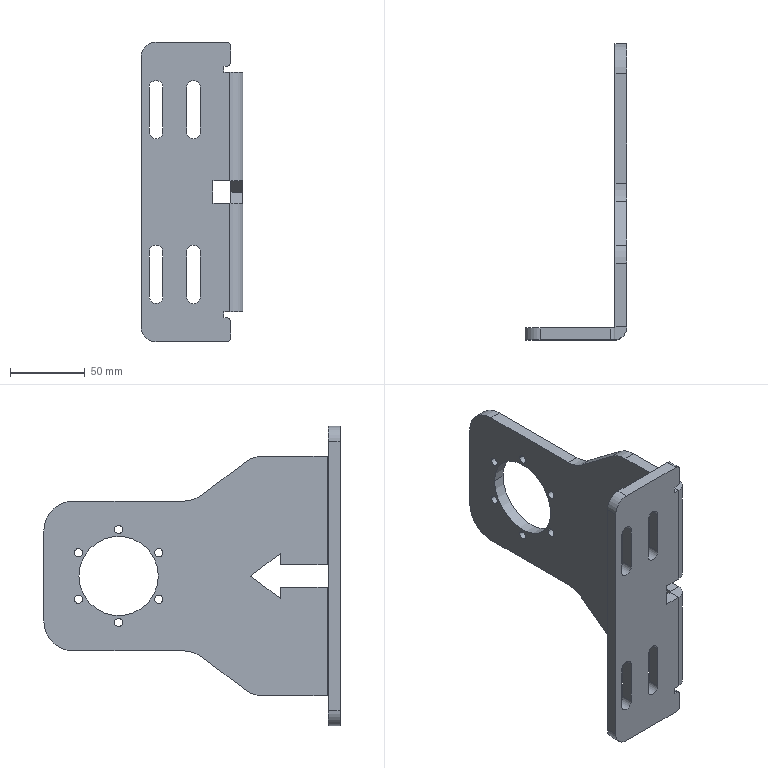Part | SolidWorks | 1 solid | 85 faces | box 68 x 198 x 200 mm | volume 249294 mm3 | plane 43 | cylinder 42 | commonest cylinder face diameters 5.5 x12 9 x12 40 x6 6 x4 1.473 x2 17.473 x2